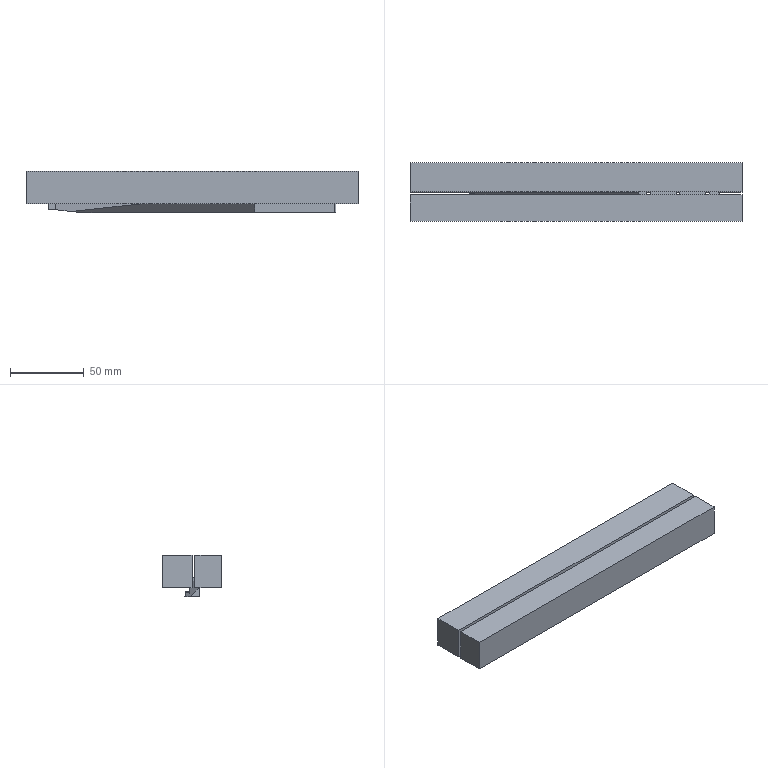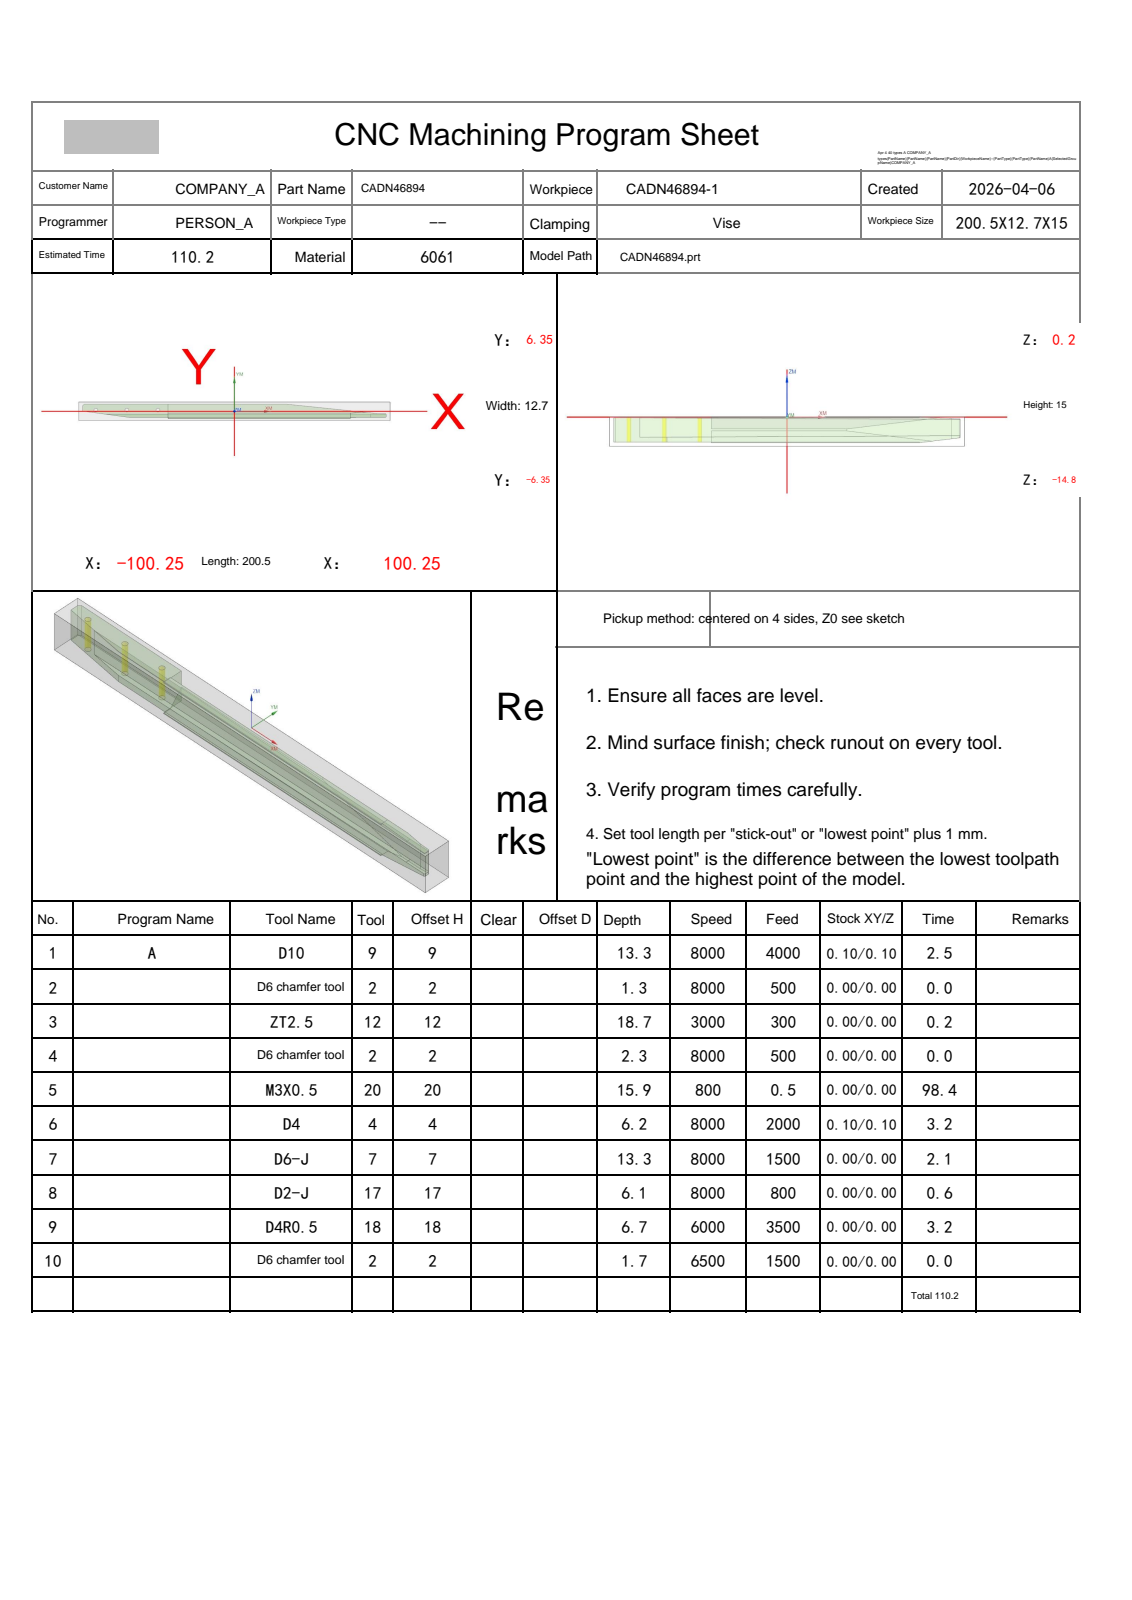NC program | NX | posted by the shop | part box 225.5 x 39.7 x 28 mm
Lines 2328 to 2996 of 2996:
N4 T02 M06
(D6 chamfer tool  D=6. R=0. H=02 ce=0.00 di=0.00)
G00 G90 G54 X-140.114 Y-11.077 M03 S6500
G43 H02 Z50.
M08
Z-.331
G01 Z-1.5 F1500.
G03 X-140.4 Y-10.877 I-1.286 J-1.532
G01 X-140.446 Y-10.847
X-140.5 Y-10.85
X-194.5
X-194.798 Y-10.811
X-195.075 Y-10.696
X-195.313 Y-10.513
X-196.313 Y-9.513
X-196.496 Y-9.275
X-196.611 Y-8.998
X-196.65 Y-8.7
Y-5.
X-196.647 Y-4.946
X-196.677 Y-4.9
G03 X-196.877 Y-4.614 I-1.732 J-1.
G01 Z-.331
G00 Z50.
G91 G28 Z0.0
M05
M09
G91 G28 Z0.0
M01
N5 T18 M06
(D4R0.5  D=4. R=0.5 H=18 ce=0.00 di=0.00)
G00 G90 G54 X-23.902 Y-.532 M03 S6000
G43 H18 Z50.
M08
Z2.989
G01 Z.154 F3500.
X-21.915 Y-.33 Z.044
X-21.845 Y-.323 Z.04
X-20.873 Y-.223 Z-.066
X-19.831 Y-.217 Z-.179
X-21.845 Y-.423 Z.04
X-21.915 Y-.43 Z.044
Y-.531
X-21.845 Y-.524 Z.04
X-18.791 Y-.212 Z-.292
X-17.768 Y-.208 Z-.403
X-21.845 Y-.624 Z.04
X-21.915 Y-.631 Z.044
Y-.732
X-21.845 Y-.725 Z.04
X-16.757 Y-.205 Z-.513
X-15.757 Y-.204 Z-.622
X-21.845 Y-.825 Z.04
X-21.915 Y-.832 Z.044
Y-.933
X-21.845 Y-.926 Z.04
X-14.757 Y-.202 Z-.731
X-13.762 Y-.201 Z-.839
X-21.845 Y-1.026 Z.04
X-21.915 Y-1.033 Z.044
Y-1.134
X-21.845 Y-1.127 Z.04
X-12.778 Y-.201 Z-.946
X-11.793 Z-1.053
X-21.845 Y-1.227 Z.04
X-21.915 Y-1.234 Z.044
Y-1.335
X-21.845 Y-1.328 Z.04
X-10.809 Y-.201 Z-1.16
X-9.824 Z-1.267
X-21.845 Y-1.428 Z.04
X-21.915 Y-1.435 Z.044
Y-1.536
X-21.845 Y-1.529 Z.04
X-8.84 Y-.201 Z-1.374
X-7.855 Z-1.481
X-21.845 Y-1.629 Z.04
X-21.915 Y-1.636 Z.044
Y-1.737
X-21.845 Y-1.73 Z.04
X-6.871 Y-.201 Z-1.588
X-5.892 Y-.202 Z-1.694
X-21.845 Y-1.83 Z.04
X-21.915 Y-1.837 Z.044
Y-1.938
X-21.845 Y-1.931 Z.04
X-4.923 Y-.203 Z-1.8
X-3.954 Y-.205 Z-1.905
X-21.845 Y-2.031 Z.04
X-21.915 Y-2.038 Z.044
Y-2.139
X-21.845 Y-2.132 Z.04
X-3.004 Y-.209 Z-2.008
X-2.062 Y-.213 Z-2.111
X-21.845 Y-2.232 Z.04
X-21.914 Y-2.239 Z.044
Y-2.34
X-21.845 Y-2.333 Z.04
X-1.14 Y-.219 Z-2.211
X-.447 Y-.226 Z-2.286
X-.247 Y-.229 Z-2.308
X-21.845 Y-2.433 Z.04
X-21.914 Y-2.44 Z.044
Y-2.541
X-21.845 Y-2.534 Z.04
X.619 Y-.241 Z-2.402
X.887 Y-.245 Z-2.431
X1.306 Y-.271 Z-2.477
X-21.845 Y-2.634 Z.04
X-21.914 Y-2.641 Z.044
Y-2.742
X-21.845 Y-2.735 Z.04
X1.493 Y-.353 Z-2.497
X1.594 Y-.412 Z-2.508
X1.629 Y-.439 Z-2.511
X-21.845 Y-2.835 Z.04
X-21.914 Y-2.842 Z.044
Y-2.943
X-21.845 Y-2.936 Z.04
X1.725 Y-.53 Z-2.522
X1.793 Y-.605 Z-2.529
X1.804 Y-.622 Z-2.53
X-21.845 Y-3.036 Z.04
X-21.914 Y-3.043 Z.044
Y-3.143
X-21.845 Y-3.136 Z.04
X1.87 Y-.716 Z-2.537
X1.935 Y-.81 Z-2.544
X-21.845 Y-3.237 Z.04
X-21.914 Y-3.244 Z.044
Y-3.344
X-21.845 Y-3.337 Z.04
X1.965 Y-.907 Z-2.548
X1.979 Y-1.006 Z-2.549
X-21.845 Y-3.438 Z.04
X-21.914 Y-3.445 Z.044
Y-3.545
X-21.845 Y-3.538 Z.04
X1.993 Y-1.105 Z-2.551
X1.998 Y-1.141 Z-2.552
X2. Y-1.205
X-21.845 Y-3.639 Z.04
X-21.914 Y-3.646 Z.044
Y-3.746
X-21.845 Y-3.739 Z.04
X2.003 Y-1.305 Z-2.552
X2.006 Y-1.405 Z-2.553
X-21.845 Y-3.84 Z.04
X-21.914 Y-3.847 Z.044
Y-3.947
X-21.845 Y-3.94 Z.04
X2.009 Y-1.505 Z-2.553
X2.01 Y-1.606
X-21.845 Y-4.041 Z.04
X-21.914 Y-4.048 Z.044
Y-4.108
X-21.911 Y-4.119
X-21.9 Y-4.123 Z.043
X-21.845 Y-4.129 Z.04
X-21.789 Y-4.136 Z.034
X2.01 Y-1.706 Z-2.553
Y-1.807
X-21.323 Y-4.188 Z-.017
X-20.857 Y-4.241 Z-.067
X2.01 Y-1.907 Z-2.553
X2.009 Y-2.008
X-20.39 Y-4.294 Z-.118
X-19.921 Y-4.347 Z-.169
X2.009 Y-2.108 Z-2.553
Y-2.209
X-19.451 Y-4.399 Z-.22
X-18.978 Y-4.452 Z-.272
X2.009 Y-2.309 Z-2.553
Y-2.41
X-18.502 Y-4.504 Z-.324
X-18.026 Y-4.555 Z-.375
X2.009 Y-2.511 Z-2.553
X2.008 Y-2.611
X-17.547 Y-4.607 Z-.427
X-17.061 Y-4.658 Z-.48
X2.008 Y-2.712 Z-2.553
X2.005 Y-2.812 Z-2.552
X-16.574 Y-4.709 Z-.533
X-16.083 Y-4.759 Z-.586
X2.001 Y-2.913 Z-2.552
X1.997 Y-3.014
X-15.587 Y-4.809 Z-.64
X-15.073 Y-4.857 Z-.696
X1.954 Y-3.119 Z-2.547
X1.904 Y-3.225 Z-2.541
X-14.559 Y-4.905 Z-.752
X-14.511 Y-4.909 Z-.757
X-14.115 Y-4.912 Z-.8
X-11.716 Y-4.683 Z-1.06
X-7.733 Y-4.274 Z-1.493
X-5.79 Y-4.076 Z-1.705
X-4.6 Y-3.957 Z-1.834
X-3.459 Y-3.851 Z-1.958
X-3.104 Y-3.836 Z-1.997
X1.854 Y-3.33 Z-2.536
X1.802 Y-3.436 Z-2.53
X-1.875 Y-3.811 Z-2.131
X-.656 Y-3.788 Z-2.263
X1.635 Y-3.554 Z-2.512
X1.46 Y-3.672 Z-2.493
X.562 Y-3.764 Z-2.396
X-1.416 Y-3.966 Z-2.181
Z1.182
G00 Z50.
G00 G90 X-63.549 Y-11.835 M03 S6000
Z50.
Z1.572
G01 Z-6.428 F3500.
X-140.689 Y-11.836 Z-6.429
X-140.971 Z-6.431
X-140.972 Y-11.765 Z-6.361
X-140.691 Z-6.358
X-62.977
X-62.867 Z-6.36
X-62.336 Y-11.71 Z-6.306
X-62.174 Y-11.694 Z-6.289
X-66.178 Z-6.287
X-140.374 Y-11.695 Z-6.288
X-140.289 Y-11.69 Z-6.282
X-140.094 Y-11.659 Z-6.252
X-139.962 Y-11.625 Z-6.218
X-61.614 Y-11.624 Z-6.219
X-61.501 Z-6.221
X-61.121 Y-11.587 Z-6.18
X-60.825 Y-11.555 Z-6.15
X-61.007 Z-6.148
X-139.741
X-139.688 Y-11.528 Z-6.121
X-139.673 Y-11.522 Z-6.114
X-139.601 Y-11.485 Z-6.077
X-60.337 Y-11.484 Z-6.078
X-60.153 Z-6.08
X-59.473 Y-11.414 Z-6.008
X-139.472 Y-11.415 Z-6.007
X-139.366 Y-11.344 Z-5.937
X-59.279
X-58.823 Z-5.94
X-58.155 Y-11.274 Z-5.867
X-139.266
Z-5.866
X-139.207 Y-11.226 Z-5.816
X-139.184 Y-11.205 Z-5.795
X-139.181 Z-5.798
X-58.048 Y-11.204
X-57.939 Z-5.8
X-57.504 Z-5.798
X-56.864 Y-11.134 Z-5.729
X-57.788 Z-5.727
X-139.107 Y-11.135 Z-5.728
X-139.09 Y-11.119 Z-5.711
X-139.043 Y-11.065 Z-5.657
X-56.206 Y-11.064
X-55.559 Y-10.993 Z-5.588
X-55.791 Z-5.586
X-138.981 Y-10.994 Z-5.587
X-138.919 Y-10.924 Z-5.517
X-55.21 Y-10.923
X-54.912 Z-5.518
X-54.521 Y-10.882 Z-5.475
X-54.27 Y-10.854 Z-5.449
X-54.643 Z-5.447
X-138.868
X-138.819 Y-10.784 Z-5.377
X-54.42
X-54.341 Z-5.378
X-53.859 Z-5.377
X-53.615 Z-5.378
X-52.976 Y-10.714 Z-5.31
X-53.192 Z-5.307
X-138.777
X-138.739 Y-10.645 Z-5.238
X-52.322 Y-10.644 Z-5.237
X-51.682 Y-10.574 Z-5.169
X-52.115 Z-5.167
X-138.701
X-138.671 Y-10.51 Z-5.103
X-138.669 Y-10.504 Z-5.097
X-51.026
X-50.743 Y-10.472 Z-5.068
X-50.384 Y-10.433 Z-5.028
X-50.427 Z-5.027
X-50.743 Z-5.028
X-50.985 Z-5.026
X-138.641 Y-10.434 Z-5.027
X-138.613 Y-10.364 Z-4.957
X-49.75 Y-10.363
X-49.734
X-49.544 Y-10.341 Z-4.938
X-49.088 Y-10.293 Z-4.887
X-49.231 Z-4.886
X-138.591
X-138.571 Y-10.223 Z-4.816
X-48.625 Y-10.222
X-48.439 Z-4.817
X-47.793 Y-10.152 Z-4.747
X-48.434 Z-4.745
X-138.552 Y-10.153
X-138.543 Y-10.119 Z-4.712
X-138.537 Y-10.083 Z-4.676
X-47.47 Y-10.082 Z-4.675
X-47.154 Z-4.678
X-46.791 Y-10.043 Z-4.638
X-46.499 Y-10.012 Z-4.606
X-47.145 Z-4.607
X-47.327 Z-4.605
X-138.526 Y-10.013 Z-4.606
X-138.514 Y-9.943 Z-4.536
X-46.038 Y-9.942
X-45.866 Z-4.539
X-45.211 Y-9.873 Z-4.466
X-138.509 Y-9.874 Z-4.467
X-138.504 Y-9.803 Z-4.396
X-44.948 Y-9.802 Z-4.395
X-44.568 Z-4.397
X-44.347 Y-9.777 Z-4.374
X-43.92 Y-9.732 Z-4.327
X-138.5 Y-9.733 Z-4.326
X-138.499 Y-9.663 Z-4.256
X-43.814 Y-9.662 Z-4.255
X-43.548 Z-4.257
X-43.273 Z-4.256
X-43.148 Y-9.647 Z-4.244
X-42.971 Y-9.63 Z-4.223
X-42.625 Y-9.592 Z-4.186
X-138.499 Y-9.593
Y-9.523 Z-4.116
X-42.231 Y-9.522 Z-4.115
X-41.983 Z-4.117
X-41.331 Y-9.452 Z-4.046
X-138.499 Z-4.045
Y-9.382 Z-3.975
X-40.89 Y-9.381
X-40.691 Z-3.977
X-40.265 Y-9.336 Z-3.93
X-40.048 Y-9.312 Z-3.907
X-40.3 Z-3.905
X-138.499 Y-9.313 Z-3.906
Y-9.243 Z-3.836
X-40.157 Y-9.242 Z-3.835
X-39.95 Z-3.836
X-39.398
X-39.15 Y-9.215 Z-3.809
X-38.94 Y-9.19 Z-3.789
X-38.765 Y-9.172 Z-3.769
X-39.017
X-39.15 Z-3.765
X-138.499 Y-9.173
Y-9.104 Z-3.697
X-38.113 Y-9.103 Z-3.696
X-37.469 Y-9.032 Z-3.627
X-38.456 Z-3.625
X-138.499 Y-9.033 Z-3.626
Y-8.963 Z-3.556
X-37.206 Y-8.962
X-36.822 Z-3.557
X-36.177 Y-8.892 Z-3.487
X-38.236 Z-3.485
X-138.499 Y-8.893 Z-3.486
Y-8.823 Z-3.416
X-35.527 Y-8.822
X-35.153 Y-8.78 Z-3.377
X-34.887 Y-8.752 Z-3.347
X-35.176 Z-3.345
X-138.499 Y-8.753 Z-3.346
Y-8.682 Z-3.275
X-34.229
X-33.592 Y-8.611 Z-3.207
X-33.733 Z-3.205
X-138.499 Y-8.612
Y-8.542 Z-3.134
X-33.128 Y-8.541
X-32.934 Z-3.135
X-32.411 Y-8.483 Z-3.079
X-32.295 Y-8.471 Z-3.066
X-32.415 Z-3.064
X-32.754 Z-3.065
X-32.984 Z-3.063
X-138.499 Z-3.064
Y-8.402 Z-2.995
X-31.737 Y-8.401
X-31.654 Z-2.997
X-30.998 Y-8.331 Z-2.925
X-138.499 Y-8.332
Y-8.261 Z-2.854
X-30.617 Y-8.26 Z-2.853
X-30.349 Z-2.855
X-29.956 Y-8.216 Z-2.813
X-29.704 Y-8.19 Z-2.785
X-31.274 Z-2.783
X-138.499 Y-8.191 Z-2.784
Y-8.121 Z-2.714
X-29.47 Y-8.12 Z-2.713
X-29.059 Z-2.715
X-28.757 Y-8.086 Z-2.683
X-28.407 Y-8.05 Z-2.644
X-138.499 Y-8.051
Y-7.981 Z-2.574
X-28.016 Y-7.98 Z-2.573
X-27.77 Z-2.576
X-27.113 Y-7.91 Z-2.503
X-138.499 Y-7.911 Z-2.504
Y-7.84 Z-2.433
X-26.57 Y-7.839
X-26.474 Z-2.435
X-25.818 Y-7.769 Z-2.363
X-138.499 Y-7.77
Y-7.7 Z-2.293
X-25.811 Y-7.699 Z-2.292
X-25.212 Z-2.294
X-25.184 Z-2.295
X-24.624 Y-7.64 Z-2.233
X-24.528 Y-7.629 Z-2.223
X-25.34 Z-2.222
X-138.499 Y-7.63
Y-7.559 Z-2.152
X-23.959 Y-7.558
X-23.88 Z-2.153
X-23.23 Y-7.488 Z-2.082
X-45.918 Z-2.081
X-138.499 Y-7.489 Z-2.082
Y-7.419 Z-2.012
X-22.879 Y-7.418
X-22.589 Z-2.013
X-21.946 Y-7.349 Z-1.943
X-22.297 Z-1.941
X-138.499 Z-1.942
Y-7.279 Z-1.872
X-21.291 Y-7.278
X-21.161 Y-7.264 Z-1.858
X-20.94 Y-7.237 Z-1.836
X-20.657 Y-7.208 Z-1.804
X-21.061
X-21.26 Z-1.801
X-138.499 Y-7.209 Z-1.802
Y-7.14 Z-1.733
X-20.004 Y-7.139 Z-1.732
X-19.363 Y-7.068 Z-1.663
X-19.773 Z-1.661
X-138.499 Y-7.069 Z-1.662
Y-6.999 Z-1.592
X-18.8 Y-6.998
X-18.717 Z-1.593
X-18.073 Y-6.928 Z-1.523
X-19.577 Z-1.521
X-138.499 Y-6.929 Z-1.522
Y-6.859 Z-1.452
X-17.563 Y-6.858
X-17.436 Z-1.455
X-17.341 Y-6.847 Z-1.446
X-16.782 Y-6.788 Z-1.384
X-17.081 Z-1.381
X-138.499 Y-6.789 Z-1.382
Y-6.719 Z-1.312
X-16.13 Y-6.718
X-15.884 Y-6.69 Z-1.287
X-15.842 Y-6.683 Z-1.281
X-15.815 Y-6.671 Z-1.271
X-15.786 Y-6.648 Z-1.248
X-15.964 Z-1.241
X-138.499 Y-6.649
Y-6.578 Z-1.171
X-15.96 Y-6.577 Z-1.17
X-15.709 Z-1.179
X-15.671 Y-6.543 Z-1.145
X-15.563 Y-6.546 Z-1.154
X-15.47 Y-6.544 Z-1.168
X-15.369 Y-6.531 Z-1.172
X-15.272 Y-6.511 Z-1.183
X-15.259 Y-6.507
X-15.371 Z-1.149
X-15.565 Z-1.116
X-15.624 Z-1.111
X-15.932 Z-1.1
X-138.5 Y-6.508 Z-1.101
Y-6.438 Z-1.031
X-15.907 Y-6.437 Z-1.03
X-15.671 Z-1.038
X-15.565 Z-1.048
X-15.376 Z-1.08
X-15.242 Z-1.122
X-15.165 Z-1.143
X-15.066 Z-1.181
X-15.025 Y-6.42 Z-1.183
X-14.917 Y-6.37 Z-1.192
X-14.912 Y-6.366
X-15.114 Z-1.098
X-15.165 Z-1.078
X-15.381 Z-1.01
X-15.565 Z-.98
X-15.717 Z-.965
X-15.882 Z-.959
X-138.5 Y-6.367 Z-.96
Y-6.314 Z-.907
X-15.862 Y-6.313 Z-.906
X-15.753 Z-.909
X-15.565 Z-.927
X-15.384 Z-.957
X-15.205 Z-1.015
X-15.165 Z-1.021
X-15.122 Z-1.036
X-14.962 Z-1.076
X-14.973 Y-6.303 Z-1.059
X-15.019 Y-6.284 Z-1.023
X-15.059 Y-6.255 Z-.977
X-15.067 Y-6.248 Z-.969
X-15.063 Y-6.245 Z-.967
X-15.186 Z-.943
X-15.255 Z-.923
X-15.322 Z-.912
X-15.389 Z-.891
X-15.462 Z-.879
X-15.565 Z-.858
X-15.797 Z-.84
X-15.838 Z-.838
X-138.5 Y-6.246 Z-.839
Y-6.206 Z-.798
X-138.503 Y-6.177 Z-.769
X-15.831 Y-6.176
X-15.565 Z-.786
X-15.387 Z-.821
X-15.315 Z-.842
X-15.281 Z-.854
X-15.186 Z-.88
X-15.202 Y-6.136 Z-.84
Y-6.13 Z-.832
X-15.197 Y-6.125 Z-.829
X-15.188 Y-6.122
X-15.148 Y-6.118 Z-.84
X-15.058 Y-6.106 Z-.866
X-15.165 Z-.82
X-15.252 Z-.789
X-15.377 Z-.751
X-15.489 Z-.728
X-15.353 Y-6.081 Z-.731
X-15.243 Y-6.054 Z-.737
X-15.18 Y-6.036 Z-.739
X-15.103 Z-.77
X-15.055 Z-.792
X-14.943 Z-.854
X-14.867 Y-5.988 Z-.847
X-14.834 Y-5.966 Z-.844
X-14.915 Z-.791
X-14.989 Z-.75
X-14.924 Y-5.937 Z-.753
X-14.843 Y-5.895 Z-.759
X-14.765 Z-.811
X-14.734 Z-.837
X-14.69 Y-5.863 Z-.835
X-14.642 Y-5.824 Z-.832
X-14.718 Z-.766
X-14.614 Y-5.754 Z-.774
X-14.559 Z-.83
X-14.481 Y-5.683 Z-.827
X-14.519 Z-.784
X-14.454 Y-5.629 Z-.792
X-14.437 Y-5.612 Z-.794
X-14.412 Z-.826
X-14.346 Y-5.542 Z-.824
X-14.362 Z-.801
X-14.295 Y-5.471 Z-.811
X-14.288 Z-.824
X-14.286
Z7.176
G00 X-15.186 Y-6.176
Z7.12
G01 Z-.88
X-15.158 Y-6.203 Z-.91
X-15.109 Y-6.197 Z-.915
X-15.057 Y-6.176 Z-.91
X-14.632 Z-.994
X-14.546 Z-1.01
X-14.497 Y-6.157 Z-1.003
X-14.381 Y-6.106 Z-.987
X-14.655 Z-.936
X-14.888 Z-.897
X-14.736 Y-6.036 Z-.885
X-14.237 Z-.968
X-14.197 Y-6.017 Z-.964
X-14.126 Y-5.966 Z-.951
X-14.606 Z-.877
X-14.49 Y-5.895 Z-.871
X-14.08 Z-.93
X-14.07 Y-5.868 Z-.923
X-14.068 Y-5.839 Z-.914
Y-5.824 Z-.91
X-14.385 Z-.867
X-14.289 Y-5.754 Z-.865
X-14.069 Z-.894
X-14.07 Y-5.683 Z-.879
X-14.203 Z-.862
X-14.118 Y-5.612
X-14.072 Z-.868
Z7.132
G00 Z50.
X-138.503 Y-6.177
Z7.231
G01 Z-.769
X-138.51 Y-6.107 Z-.7
X-15.849 Y-6.106 Z-.699
X-15.797 Z-.701
X-15.791 Y-6.036 Z-.632
X-15.867 Z-.629
X-138.527 Y-6.037 Z-.63
X-138.558 Y-5.977 Z-.57
X-138.562 Y-5.967 Z-.559
X-16.854 Y-5.966
X-16.764 Z-.56
X-16.584 Z-.559
X-16.144
X-15.907 Z-.561
X-16.381 Y-5.916 Z-.509
X-16.565 Y-5.895 Z-.491
X-16.764 Z-.493
X-16.998 Z-.488
X-138.611 Y-5.896 Z-.489
X-138.664 Y-5.828 Z-.421
X-138.669 Y-5.825 Z-.418
X-17.236 Y-5.824
X-17.563 Y-5.788 Z-.384
X-17.894 Y-5.754 Z-.348
X-18.517 Z-.347
X-18.763 Z-.348
X-20.76 Z-.347
X-138.788 Y-5.755
X-138.833 Y-5.732 Z-.329
X-138.866 Y-5.722 Z-.317
X-138.918 Y-5.717 Z-.31
X-139.101 Y-5.707 Z-.3
X-140.955
X-140.979 Y-5.701 Z-.295
X-140.986 Y-5.684 Z-.28
X-140.689 Z-.277
X-19.032 Y-5.683 Z-.276
X-18.763 Z-.279
X-18.556 Z-.278
X-18.866 Y-5.65 Z-.245
X-19.234 Y-5.613 Z-.206
X-140.689
X-140.982 Z-.209
X-140.979 Y-5.543 Z-.138
X-140.689 Z-.136
X-19.912 Y-5.542 Z-.135
X-20.362 Y-5.494 Z-.09
X-20.586 Y-5.471 Z-.065
X-140.689 Y-5.472
X-140.976 Z-.068
X-140.974 Y-5.401 Z.003
X-140.689 Z.006
X-21.288 Y-5.4
X-21.561 Y-5.373 Z.032
X-22.01 Y-5.33 Z.077
X-140.689 Y-5.331 Z.076
X-140.972 Z.074
X-140.97 Y-5.26 Z.144
X-140.689 Z.147
X-22.723 Y-5.259
Z8.147
G00 Z50.
M05
M09
G91 G28 Z0.0
G91 G28 Y0.0
M30
%